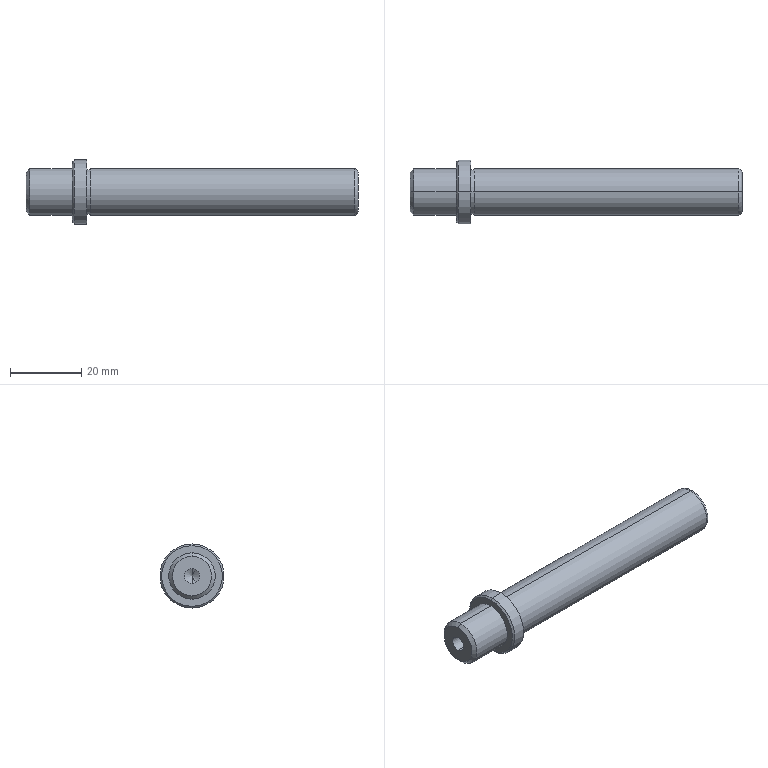Part | SolidWorks | features Chamfer 2, Fillet 1, HoleWzd 1, Revolution 1 | 1 solid | 23 faces | box 93 x 18 x 18 mm | volume 12586 mm3 | cylinder 10 | cone 6 | plane 5 | torus 2 | commonest cylinder face diameters 13 x4 4.2 x2 12.5 x2 18 x2
STEP:
#1=CARTESIAN_POINT('',(14.,0.,-2.1));
#2=VERTEX_POINT('',#1);
#3=CARTESIAN_POINT('',(14.,0.,2.1));
#4=VERTEX_POINT('',#3);
#5=CARTESIAN_POINT('',(14.,0.,0.));
#6=DIRECTION('',(-1.,0.,0.));
#7=DIRECTION('',(0.,0.,1.));
#8=AXIS2_PLACEMENT_3D('',#5,#6,#7);
#9=CIRCLE('',#8,2.1);
#10=EDGE_CURVE('',#2,#4,#9,.T.);
#11=ORIENTED_EDGE('',*,*,#10,.F.);
#12=CARTESIAN_POINT('',(0.,0.,-2.1));
#13=VERTEX_POINT('',#12);
#14=CARTESIAN_POINT('',(0.,0.,-2.1));
#15=DIRECTION('',(-1.,0.,0.));
#16=VECTOR('',#15,1000.);
#17=LINE('',#14,#16);
#18=EDGE_CURVE('',#2,#13,#17,.T.);
#19=ORIENTED_EDGE('',*,*,#18,.T.);
#20=CARTESIAN_POINT('',(0.,0.,2.1));
#21=VERTEX_POINT('',#20);
#22=CARTESIAN_POINT('',(0.,0.,0.));
#23=DIRECTION('',(-1.,0.,0.));
#24=DIRECTION('',(0.,0.,1.));
#25=AXIS2_PLACEMENT_3D('',#22,#23,#24);
#26=CIRCLE('',#25,2.1);
#27=EDGE_CURVE('',#13,#21,#26,.T.);
#28=ORIENTED_EDGE('',*,*,#27,.T.);
#29=CARTESIAN_POINT('',(0.,0.,2.1));
#30=DIRECTION('',(-1.,0.,0.));
#31=VECTOR('',#30,1000.);
#32=LINE('',#29,#31);
#33=EDGE_CURVE('',#4,#21,#32,.T.);
#34=ORIENTED_EDGE('',*,*,#33,.F.);
#35=EDGE_LOOP('',(#11,#19,#28,#34));
#36=FACE_OUTER_BOUND('',#35,.T.);
#37=CARTESIAN_POINT('',(0.,0.,0.));
#38=DIRECTION('',(-1.,0.,0.));
#39=DIRECTION('',(0.,0.,1.));
#40=AXIS2_PLACEMENT_3D('',#37,#38,#39);
#41=CYLINDRICAL_SURFACE('',#40,2.1);
#42=ADVANCED_FACE('',(#36),#41,.F.);
#43=CARTESIAN_POINT('',(15.262,0.,0.));
#44=VERTEX_POINT('',#43);
#45=CARTESIAN_POINT('',(14.,0.,2.1));
#46=DIRECTION('',(-0.515,0.,0.8572));
#47=VECTOR('',#46,1000.);
#48=LINE('',#45,#47);
#49=EDGE_CURVE('',#44,#4,#48,.T.);
#50=ORIENTED_EDGE('',*,*,#49,.F.);
#51=CARTESIAN_POINT('',(14.,0.,-2.1));
#52=DIRECTION('',(-0.515,0.,-0.8572));
#53=VECTOR('',#52,1000.);
#54=LINE('',#51,#53);
#55=EDGE_CURVE('',#44,#2,#54,.T.);
#56=ORIENTED_EDGE('',*,*,#55,.T.);
#57=ORIENTED_EDGE('',*,*,#10,.T.);
#58=EDGE_LOOP('',(#50,#56,#57));
#59=FACE_OUTER_BOUND('',#58,.T.);
#60=CARTESIAN_POINT('',(14.,0.,0.));
#61=DIRECTION('',(-1.,0.,0.));
#62=DIRECTION('',(0.,0.,1.));
#63=AXIS2_PLACEMENT_3D('',#60,#61,#62);
#64=CONICAL_SURFACE('',#63,2.1,1.03);
#65=ADVANCED_FACE('',(#59),#64,.F.);
#66=CARTESIAN_POINT('',(0.,0.,5.5));
#67=VERTEX_POINT('',#66);
#68=CARTESIAN_POINT('',(0.,0.,-5.5));
#69=VERTEX_POINT('',#68);
#70=CARTESIAN_POINT('',(0.,0.,0.));
#71=DIRECTION('',(-1.,0.,0.));
#72=DIRECTION('',(0.,0.,-1.));
#73=AXIS2_PLACEMENT_3D('',#70,#71,#72);
#74=CIRCLE('',#73,5.5);
#75=EDGE_CURVE('',#67,#69,#74,.T.);
#76=ORIENTED_EDGE('',*,*,#75,.F.);
#77=CARTESIAN_POINT('',(1.,0.,6.5));
#78=VERTEX_POINT('',#77);
#79=CARTESIAN_POINT('',(0.,0.,5.5));
#80=DIRECTION('',(0.7071,0.,0.7071));
#81=VECTOR('',#80,1000.);
#82=LINE('',#79,#81);
#83=EDGE_CURVE('',#67,#78,#82,.T.);
#84=ORIENTED_EDGE('',*,*,#83,.T.);
#85=CARTESIAN_POINT('',(1.,0.,-6.5));
#86=VERTEX_POINT('',#85);
#87=CARTESIAN_POINT('',(1.,0.,0.));
#88=DIRECTION('',(1.,0.,0.));
#89=DIRECTION('',(0.,0.,-1.));
#90=AXIS2_PLACEMENT_3D('',#87,#88,#89);
#91=CIRCLE('',#90,6.5);
#92=EDGE_CURVE('',#86,#78,#91,.T.);
#93=ORIENTED_EDGE('',*,*,#92,.F.);
#94=CARTESIAN_POINT('',(0.,0.,-5.5));
#95=DIRECTION('',(0.7071,0.,-0.7071));
#96=VECTOR('',#95,1000.);
#97=LINE('',#94,#96);
#98=EDGE_CURVE('',#69,#86,#97,.T.);
#99=ORIENTED_EDGE('',*,*,#98,.F.);
#100=EDGE_LOOP('',(#76,#84,#93,#99));
#101=FACE_OUTER_BOUND('',#100,.T.);
#102=CARTESIAN_POINT('',(0.,0.,0.));
#103=DIRECTION('',(1.,0.,0.));
#104=DIRECTION('',(0.,0.,-1.));
#105=AXIS2_PLACEMENT_3D('',#102,#103,#104);
#106=CONICAL_SURFACE('',#105,5.5,0.7854);
#107=ADVANCED_FACE('',(#101),#106,.T.);
#108=CARTESIAN_POINT('',(13.,0.,8.5));
#109=VERTEX_POINT('',#108);
#110=CARTESIAN_POINT('',(13.,0.,-8.5));
#111=VERTEX_POINT('',#110);
#112=CARTESIAN_POINT('',(13.,0.,0.));
#113=DIRECTION('',(-1.,0.,0.));
#114=DIRECTION('',(0.,0.,-1.));
#115=AXIS2_PLACEMENT_3D('',#112,#113,#114);
#116=CIRCLE('',#115,8.5);
#117=EDGE_CURVE('',#109,#111,#116,.T.);
#118=ORIENTED_EDGE('',*,*,#117,.F.);
#119=CARTESIAN_POINT('',(13.5,0.,9.));
#120=VERTEX_POINT('',#119);
#121=CARTESIAN_POINT('',(13.,0.,8.5));
#122=DIRECTION('',(0.7071,0.,0.7071));
#123=VECTOR('',#122,1000.);
#124=LINE('',#121,#123);
#125=EDGE_CURVE('',#109,#120,#124,.T.);
#126=ORIENTED_EDGE('',*,*,#125,.T.);
#127=CARTESIAN_POINT('',(13.5,0.,-9.));
#128=VERTEX_POINT('',#127);
#129=CARTESIAN_POINT('',(13.5,0.,0.));
#130=DIRECTION('',(1.,0.,0.));
#131=DIRECTION('',(0.,0.,-1.));
#132=AXIS2_PLACEMENT_3D('',#129,#130,#131);
#133=CIRCLE('',#132,9.);
#134=EDGE_CURVE('',#128,#120,#133,.T.);
#135=ORIENTED_EDGE('',*,*,#134,.F.);
#136=CARTESIAN_POINT('',(13.,0.,-8.5));
#137=DIRECTION('',(0.7071,0.,-0.7071));
#138=VECTOR('',#137,1000.);
#139=LINE('',#136,#138);
#140=EDGE_CURVE('',#111,#128,#139,.T.);
#141=ORIENTED_EDGE('',*,*,#140,.F.);
#142=EDGE_LOOP('',(#118,#126,#135,#141));
#143=FACE_OUTER_BOUND('',#142,.T.);
#144=CARTESIAN_POINT('',(13.,0.,0.));
#145=DIRECTION('',(1.,0.,0.));
#146=DIRECTION('',(0.,0.,-1.));
#147=AXIS2_PLACEMENT_3D('',#144,#145,#146);
#148=CONICAL_SURFACE('',#147,8.5,0.7854);
#149=ADVANCED_FACE('',(#143),#148,.T.);
#150=CARTESIAN_POINT('',(93.,0.,-5.5));
#151=VERTEX_POINT('',#150);
#152=CARTESIAN_POINT('',(93.,0.,5.5));
#153=VERTEX_POINT('',#152);
#154=CARTESIAN_POINT('',(93.,0.,0.));
#155=DIRECTION('',(1.,0.,0.));
#156=DIRECTION('',(0.,0.,1.));
#157=AXIS2_PLACEMENT_3D('',#154,#155,#156);
#158=CIRCLE('',#157,5.5);
#159=EDGE_CURVE('',#151,#153,#158,.T.);
#160=ORIENTED_EDGE('',*,*,#159,.F.);
#161=CARTESIAN_POINT('',(92.,0.,-6.5));
#162=VERTEX_POINT('',#161);
#163=CARTESIAN_POINT('',(92.,0.,-5.5));
#164=DIRECTION('',(0.,1.,0.));
#165=DIRECTION('',(0.,0.,1.));
#166=AXIS2_PLACEMENT_3D('',#163,#164,#165);
#167=CIRCLE('',#166,1.);
#168=EDGE_CURVE('',#151,#162,#167,.T.);
#169=ORIENTED_EDGE('',*,*,#168,.T.);
#170=CARTESIAN_POINT('',(92.,0.,6.5));
#171=VERTEX_POINT('',#170);
#172=CARTESIAN_POINT('',(92.,0.,0.));
#173=DIRECTION('',(-1.,0.,0.));
#174=DIRECTION('',(0.,0.,1.));
#175=AXIS2_PLACEMENT_3D('',#172,#173,#174);
#176=CIRCLE('',#175,6.5);
#177=EDGE_CURVE('',#171,#162,#176,.T.);
#178=ORIENTED_EDGE('',*,*,#177,.F.);
#179=CARTESIAN_POINT('',(92.,0.,5.5));
#180=DIRECTION('',(0.,-1.,0.));
#181=DIRECTION('',(0.,0.,-1.));
#182=AXIS2_PLACEMENT_3D('',#179,#180,#181);
#183=CIRCLE('',#182,1.);
#184=EDGE_CURVE('',#153,#171,#183,.T.);
#185=ORIENTED_EDGE('',*,*,#184,.F.);
#186=EDGE_LOOP('',(#160,#169,#178,#185));
#187=FACE_OUTER_BOUND('',#186,.T.);
#188=CARTESIAN_POINT('',(92.,0.,0.));
#189=DIRECTION('',(-1.,0.,0.));
#190=DIRECTION('',(0.,0.,1.));
#191=AXIS2_PLACEMENT_3D('',#188,#189,#190);
#192=TOROIDAL_SURFACE('',#191,5.5,1.);
#193=ADVANCED_FACE('',(#187),#192,.T.);
#194=CARTESIAN_POINT('',(17.,0.,9.));
#195=VERTEX_POINT('',#194);
#196=CARTESIAN_POINT('',(17.,0.,-9.));
#197=VERTEX_POINT('',#196);
#198=CARTESIAN_POINT('',(17.,0.,0.));
#199=DIRECTION('',(-1.,0.,0.));
#200=DIRECTION('',(0.,0.,1.));
#201=AXIS2_PLACEMENT_3D('',#198,#199,#200);
#202=CIRCLE('',#201,9.);
#203=EDGE_CURVE('',#195,#197,#202,.T.);
#204=ORIENTED_EDGE('',*,*,#203,.T.);
#205=CARTESIAN_POINT('',(0.,0.,-9.));
#206=DIRECTION('',(-1.,0.,0.));
#207=VECTOR('',#206,1000.);
#208=LINE('',#205,#207);
#209=EDGE_CURVE('',#197,#128,#208,.T.);
#210=ORIENTED_EDGE('',*,*,#209,.T.);
#211=ORIENTED_EDGE('',*,*,#134,.T.);
#212=CARTESIAN_POINT('',(0.,0.,9.));
#213=DIRECTION('',(-1.,0.,0.));
#214=VECTOR('',#213,1000.);
#215=LINE('',#212,#214);
#216=EDGE_CURVE('',#195,#120,#215,.T.);
#217=ORIENTED_EDGE('',*,*,#216,.F.);
#218=EDGE_LOOP('',(#204,#210,#211,#217));
#219=FACE_OUTER_BOUND('',#218,.T.);
#220=CARTESIAN_POINT('',(0.,0.,0.));
#221=DIRECTION('',(-1.,0.,0.));
#222=DIRECTION('',(0.,0.,1.));
#223=AXIS2_PLACEMENT_3D('',#220,#221,#222);
#224=CYLINDRICAL_SURFACE('',#223,9.);
#225=ADVANCED_FACE('',(#219),#224,.T.);
#226=CARTESIAN_POINT('',(18.,0.,6.25));
#227=VERTEX_POINT('',#226);
#228=CARTESIAN_POINT('',(18.,0.,-6.25));
#229=VERTEX_POINT('',#228);
#230=CARTESIAN_POINT('',(18.,0.,0.));
#231=DIRECTION('',(-1.,0.,0.));
#232=DIRECTION('',(0.,0.,1.));
#233=AXIS2_PLACEMENT_3D('',#230,#231,#232);
#234=CIRCLE('',#233,6.25);
#235=EDGE_CURVE('',#227,#229,#234,.T.);
#236=ORIENTED_EDGE('',*,*,#235,.T.);
#237=CARTESIAN_POINT('',(17.,0.,-6.25));
#238=VERTEX_POINT('',#237);
#239=CARTESIAN_POINT('',(0.,0.,-6.25));
#240=DIRECTION('',(-1.,0.,0.));
#241=VECTOR('',#240,1000.);
#242=LINE('',#239,#241);
#243=EDGE_CURVE('',#229,#238,#242,.T.);
#244=ORIENTED_EDGE('',*,*,#243,.T.);
#245=CARTESIAN_POINT('',(17.,0.,6.25));
#246=VERTEX_POINT('',#245);
#247=CARTESIAN_POINT('',(17.,0.,0.));
#248=DIRECTION('',(-1.,0.,0.));
#249=DIRECTION('',(0.,0.,1.));
#250=AXIS2_PLACEMENT_3D('',#247,#248,#249);
#251=CIRCLE('',#250,6.25);
#252=EDGE_CURVE('',#246,#238,#251,.T.);
#253=ORIENTED_EDGE('',*,*,#252,.F.);
#254=CARTESIAN_POINT('',(0.,0.,6.25));
#255=DIRECTION('',(-1.,0.,0.));
#256=VECTOR('',#255,1000.);
#257=LINE('',#254,#256);
#258=EDGE_CURVE('',#227,#246,#257,.T.);
#259=ORIENTED_EDGE('',*,*,#258,.F.);
#260=EDGE_LOOP('',(#236,#244,#253,#259));
#261=FACE_OUTER_BOUND('',#260,.T.);
#262=CARTESIAN_POINT('',(0.,0.,0.));
#263=DIRECTION('',(-1.,0.,0.));
#264=DIRECTION('',(0.,0.,1.));
#265=AXIS2_PLACEMENT_3D('',#262,#263,#264);
#266=CYLINDRICAL_SURFACE('',#265,6.25);
#267=ADVANCED_FACE('',(#261),#266,.T.);
#268=ORIENTED_EDGE('',*,*,#177,.T.);
#269=CARTESIAN_POINT('',(18.,0.,-6.5));
#270=VERTEX_POINT('',#269);
#271=CARTESIAN_POINT('',(0.,0.,-6.5));
#272=DIRECTION('',(-1.,0.,0.));
#273=VECTOR('',#272,1000.);
#274=LINE('',#271,#273);
#275=EDGE_CURVE('',#162,#270,#274,.T.);
#276=ORIENTED_EDGE('',*,*,#275,.T.);
#277=CARTESIAN_POINT('',(18.,0.,6.5));
#278=VERTEX_POINT('',#277);
#279=CARTESIAN_POINT('',(18.,0.,0.));
#280=DIRECTION('',(-1.,0.,0.));
#281=DIRECTION('',(0.,0.,1.));
#282=AXIS2_PLACEMENT_3D('',#279,#280,#281);
#283=CIRCLE('',#282,6.5);
#284=EDGE_CURVE('',#278,#270,#283,.T.);
#285=ORIENTED_EDGE('',*,*,#284,.F.);
#286=CARTESIAN_POINT('',(0.,0.,6.5));
#287=DIRECTION('',(-1.,0.,0.));
#288=VECTOR('',#287,1000.);
#289=LINE('',#286,#288);
#290=EDGE_CURVE('',#171,#278,#289,.T.);
#291=ORIENTED_EDGE('',*,*,#290,.F.);
#292=EDGE_LOOP('',(#268,#276,#285,#291));
#293=FACE_OUTER_BOUND('',#292,.T.);
#294=CARTESIAN_POINT('',(0.,0.,0.));
#295=DIRECTION('',(-1.,0.,0.));
#296=DIRECTION('',(0.,0.,1.));
#297=AXIS2_PLACEMENT_3D('',#294,#295,#296);
#298=CYLINDRICAL_SURFACE('',#297,6.5);
#299=ADVANCED_FACE('',(#293),#298,.T.);
#300=CARTESIAN_POINT('',(13.,0.,6.5));
#301=VERTEX_POINT('',#300);
#302=CARTESIAN_POINT('',(13.,0.,-6.5));
#303=VERTEX_POINT('',#302);
#304=CARTESIAN_POINT('',(13.,0.,0.));
#305=DIRECTION('',(-1.,0.,0.));
#306=DIRECTION('',(0.,0.,1.));
#307=AXIS2_PLACEMENT_3D('',#304,#305,#306);
#308=CIRCLE('',#307,6.5);
#309=EDGE_CURVE('',#301,#303,#308,.T.);
#310=ORIENTED_EDGE('',*,*,#309,.T.);
#311=CARTESIAN_POINT('',(0.,0.,-6.5));
#312=DIRECTION('',(-1.,0.,0.));
#313=VECTOR('',#312,1000.);
#314=LINE('',#311,#313);
#315=EDGE_CURVE('',#303,#86,#314,.T.);
#316=ORIENTED_EDGE('',*,*,#315,.T.);
#317=ORIENTED_EDGE('',*,*,#92,.T.);
#318=CARTESIAN_POINT('',(0.,0.,6.5));
#319=DIRECTION('',(-1.,0.,0.));
#320=VECTOR('',#319,1000.);
#321=LINE('',#318,#320);
#322=EDGE_CURVE('',#301,#78,#321,.T.);
#323=ORIENTED_EDGE('',*,*,#322,.F.);
#324=EDGE_LOOP('',(#310,#316,#317,#323));
#325=FACE_OUTER_BOUND('',#324,.T.);
#326=CARTESIAN_POINT('',(0.,0.,0.));
#327=DIRECTION('',(-1.,0.,0.));
#328=DIRECTION('',(0.,0.,1.));
#329=AXIS2_PLACEMENT_3D('',#326,#327,#328);
#330=CYLINDRICAL_SURFACE('',#329,6.5);
#331=ADVANCED_FACE('',(#325),#330,.T.);
#332=ORIENTED_EDGE('',*,*,#315,.F.);
#333=CARTESIAN_POINT('',(13.,0.,0.));
#334=DIRECTION('',(-1.,0.,0.));
#335=DIRECTION('',(0.,0.,1.));
#336=AXIS2_PLACEMENT_3D('',#333,#334,#335);
#337=CIRCLE('',#336,6.5);
#338=EDGE_CURVE('',#303,#301,#337,.T.);
#339=ORIENTED_EDGE('',*,*,#338,.T.);
#340=ORIENTED_EDGE('',*,*,#322,.T.);
#341=CARTESIAN_POINT('',(1.,0.,0.));
#342=DIRECTION('',(1.,0.,0.));
#343=DIRECTION('',(0.,0.,-1.));
#344=AXIS2_PLACEMENT_3D('',#341,#342,#343);
#345=CIRCLE('',#344,6.5);
#346=EDGE_CURVE('',#78,#86,#345,.T.);
#347=ORIENTED_EDGE('',*,*,#346,.T.);
#348=EDGE_LOOP('',(#332,#339,#340,#347));
#349=FACE_OUTER_BOUND('',#348,.T.);
#350=CARTESIAN_POINT('',(0.,0.,0.));
#351=DIRECTION('',(-1.,0.,0.));
#352=DIRECTION('',(0.,0.,1.));
#353=AXIS2_PLACEMENT_3D('',#350,#351,#352);
#354=CYLINDRICAL_SURFACE('',#353,6.5);
#355=ADVANCED_FACE('',(#349),#354,.T.);
#356=CARTESIAN_POINT('',(0.,0.,0.));
#357=DIRECTION('',(-1.,0.,0.));
#358=DIRECTION('',(0.,0.,1.));
#359=AXIS2_PLACEMENT_3D('',#356,#357,#358);
#360=CIRCLE('',#359,2.1);
#361=EDGE_CURVE('',#21,#13,#360,.T.);
#362=ORIENTED_EDGE('',*,*,#361,.F.);
#363=ORIENTED_EDGE('',*,*,#27,.F.);
#364=EDGE_LOOP('',(#362,#363));
#365=FACE_BOUND('',#364,.T.);
#366=CARTESIAN_POINT('',(0.,0.,0.));
#367=DIRECTION('',(-1.,0.,0.));
#368=DIRECTION('',(0.,0.,-1.));
#369=AXIS2_PLACEMENT_3D('',#366,#367,#368);
#370=CIRCLE('',#369,5.5);
#371=EDGE_CURVE('',#69,#67,#370,.T.);
#372=ORIENTED_EDGE('',*,*,#371,.T.);
#373=ORIENTED_EDGE('',*,*,#75,.T.);
#374=EDGE_LOOP('',(#372,#373));
#375=FACE_OUTER_BOUND('',#374,.T.);
#376=CARTESIAN_POINT('',(0.,6.5,0.));
#377=DIRECTION('',(1.,0.,0.));
#378=DIRECTION('',(0.,0.,-1.));
#379=AXIS2_PLACEMENT_3D('',#376,#377,#378);
#380=PLANE('',#379);
#381=ADVANCED_FACE('',(#365,#375),#380,.F.);
#382=CARTESIAN_POINT('',(93.,0.,0.));
#383=DIRECTION('',(1.,0.,0.));
#384=DIRECTION('',(0.,0.,1.));
#385=AXIS2_PLACEMENT_3D('',#382,#383,#384);
#386=CIRCLE('',#385,5.5);
#387=EDGE_CURVE('',#153,#151,#386,.T.);
#388=ORIENTED_EDGE('',*,*,#387,.T.);
#389=ORIENTED_EDGE('',*,*,#159,.T.);
#390=EDGE_LOOP('',(#388,#389));
#391=FACE_OUTER_BOUND('',#390,.T.);
#392=CARTESIAN_POINT('',(93.,6.5,0.));
#393=DIRECTION('',(-1.,0.,0.));
#394=DIRECTION('',(0.,0.,1.));
#395=AXIS2_PLACEMENT_3D('',#392,#393,#394);
#396=PLANE('',#395);
#397=ADVANCED_FACE('',(#391),#396,.F.);
#398=ORIENTED_EDGE('',*,*,#275,.F.);
#399=CARTESIAN_POINT('',(92.,0.,0.));
#400=DIRECTION('',(-1.,0.,0.));
#401=DIRECTION('',(0.,0.,1.));
#402=AXIS2_PLACEMENT_3D('',#399,#400,#401);
#403=CIRCLE('',#402,6.5);
#404=EDGE_CURVE('',#162,#171,#403,.T.);
#405=ORIENTED_EDGE('',*,*,#404,.T.);
#406=ORIENTED_EDGE('',*,*,#290,.T.);
#407=CARTESIAN_POINT('',(18.,0.,0.));
#408=DIRECTION('',(-1.,0.,0.));
#409=DIRECTION('',(0.,0.,1.));
#410=AXIS2_PLACEMENT_3D('',#407,#408,#409);
#411=CIRCLE('',#410,6.5);
#412=EDGE_CURVE('',#270,#278,#411,.T.);
#413=ORIENTED_EDGE('',*,*,#412,.F.);
#414=EDGE_LOOP('',(#398,#405,#406,#413));
#415=FACE_OUTER_BOUND('',#414,.T.);
#416=CARTESIAN_POINT('',(0.,0.,0.));
#417=DIRECTION('',(-1.,0.,0.));
#418=DIRECTION('',(0.,0.,1.));
#419=AXIS2_PLACEMENT_3D('',#416,#417,#418);
#420=CYLINDRICAL_SURFACE('',#419,6.5);
#421=ADVANCED_FACE('',(#415),#420,.T.);
#422=ORIENTED_EDGE('',*,*,#235,.F.);
#423=CARTESIAN_POINT('',(18.,0.,0.));
#424=DIRECTION('',(-1.,0.,0.));
#425=DIRECTION('',(0.,0.,1.));
#426=AXIS2_PLACEMENT_3D('',#423,#424,#425);
#427=CIRCLE('',#426,6.25);
#428=EDGE_CURVE('',#229,#227,#427,.T.);
#429=ORIENTED_EDGE('',*,*,#428,.F.);
#430=EDGE_LOOP('',(#422,#429));
#431=FACE_BOUND('',#430,.T.);
#432=ORIENTED_EDGE('',*,*,#284,.T.);
#433=ORIENTED_EDGE('',*,*,#412,.T.);
#434=EDGE_LOOP('',(#432,#433));
#435=FACE_OUTER_BOUND('',#434,.T.);
#436=CARTESIAN_POINT('',(18.,6.25,0.));
#437=DIRECTION('',(1.,0.,0.));
#438=DIRECTION('',(0.,0.,-1.));
#439=AXIS2_PLACEMENT_3D('',#436,#437,#438);
#440=PLANE('',#439);
#441=ADVANCED_FACE('',(#431,#435),#440,.F.);
#442=ORIENTED_EDGE('',*,*,#243,.F.);
#443=ORIENTED_EDGE('',*,*,#428,.T.);
#444=ORIENTED_EDGE('',*,*,#258,.T.);
#445=CARTESIAN_POINT('',(17.,0.,0.));
#446=DIRECTION('',(-1.,0.,0.));
#447=DIRECTION('',(0.,0.,1.));
#448=AXIS2_PLACEMENT_3D('',#445,#446,#447);
#449=CIRCLE('',#448,6.25);
#450=EDGE_CURVE('',#238,#246,#449,.T.);
#451=ORIENTED_EDGE('',*,*,#450,.F.);
#452=EDGE_LOOP('',(#442,#443,#444,#451));
#453=FACE_OUTER_BOUND('',#452,.T.);
#454=CARTESIAN_POINT('',(0.,0.,0.));
#455=DIRECTION('',(-1.,0.,0.));
#456=DIRECTION('',(0.,0.,1.));
#457=AXIS2_PLACEMENT_3D('',#454,#455,#456);
#458=CYLINDRICAL_SURFACE('',#457,6.25);
#459=ADVANCED_FACE('',(#453),#458,.T.);
#460=ORIENTED_EDGE('',*,*,#203,.F.);
#461=CARTESIAN_POINT('',(17.,0.,0.));
#462=DIRECTION('',(-1.,0.,0.));
#463=DIRECTION('',(0.,0.,1.));
#464=AXIS2_PLACEMENT_3D('',#461,#462,#463);
#465=CIRCLE('',#464,9.);
#466=EDGE_CURVE('',#197,#195,#465,.T.);
#467=ORIENTED_EDGE('',*,*,#466,.F.);
#468=EDGE_LOOP('',(#460,#467));
#469=FACE_OUTER_BOUND('',#468,.T.);
#470=ORIENTED_EDGE('',*,*,#252,.T.);
#471=ORIENTED_EDGE('',*,*,#450,.T.);
#472=EDGE_LOOP('',(#470,#471));
#473=FACE_BOUND('',#472,.T.);
#474=CARTESIAN_POINT('',(17.,9.,0.));
#475=DIRECTION('',(-1.,0.,0.));
#476=DIRECTION('',(0.,0.,1.));
#477=AXIS2_PLACEMENT_3D('',#474,#475,#476);
#478=PLANE('',#477);
#479=ADVANCED_FACE('',(#469,#473),#478,.F.);
#480=ORIENTED_EDGE('',*,*,#209,.F.);
#481=ORIENTED_EDGE('',*,*,#466,.T.);
#482=ORIENTED_EDGE('',*,*,#216,.T.);
#483=CARTESIAN_POINT('',(13.5,0.,0.));
#484=DIRECTION('',(1.,0.,0.));
#485=DIRECTION('',(0.,0.,-1.));
#486=AXIS2_PLACEMENT_3D('',#483,#484,#485);
#487=CIRCLE('',#486,9.);
#488=EDGE_CURVE('',#120,#128,#487,.T.);
#489=ORIENTED_EDGE('',*,*,#488,.T.);
#490=EDGE_LOOP('',(#480,#481,#482,#489));
#491=FACE_OUTER_BOUND('',#490,.T.);
#492=CARTESIAN_POINT('',(0.,0.,0.));
#493=DIRECTION('',(-1.,0.,0.));
#494=DIRECTION('',(0.,0.,1.));
#495=AXIS2_PLACEMENT_3D('',#492,#493,#494);
#496=CYLINDRICAL_SURFACE('',#495,9.);
#497=ADVANCED_FACE('',(#491),#496,.T.);
#498=CARTESIAN_POINT('',(13.,0.,0.));
#499=DIRECTION('',(-1.,0.,0.));
#500=DIRECTION('',(0.,0.,-1.));
#501=AXIS2_PLACEMENT_3D('',#498,#499,#500);
#502=CIRCLE('',#501,8.5);
#503=EDGE_CURVE('',#111,#109,#502,.T.);
#504=ORIENTED_EDGE('',*,*,#503,.T.);
#505=ORIENTED_EDGE('',*,*,#117,.T.);
#506=EDGE_LOOP('',(#504,#505));
#507=FACE_OUTER_BOUND('',#506,.T.);
#508=ORIENTED_EDGE('',*,*,#309,.F.);
#509=ORIENTED_EDGE('',*,*,#338,.F.);
#510=EDGE_LOOP('',(#508,#509));
#511=FACE_BOUND('',#510,.T.);
#512=CARTESIAN_POINT('',(13.,6.5,0.));
#513=DIRECTION('',(1.,0.,0.));
#514=DIRECTION('',(0.,0.,-1.));
#515=AXIS2_PLACEMENT_3D('',#512,#513,#514);
#516=PLANE('',#515);
#517=ADVANCED_FACE('',(#507,#511),#516,.F.);
#518=ORIENTED_EDGE('',*,*,#168,.F.);
#519=ORIENTED_EDGE('',*,*,#387,.F.);
#520=ORIENTED_EDGE('',*,*,#184,.T.);
#521=ORIENTED_EDGE('',*,*,#404,.F.);
#522=EDGE_LOOP('',(#518,#519,#520,#521));
#523=FACE_OUTER_BOUND('',#522,.T.);
#524=CARTESIAN_POINT('',(92.,0.,0.));
#525=DIRECTION('',(-1.,0.,0.));
#526=DIRECTION('',(0.,0.,1.));
#527=AXIS2_PLACEMENT_3D('',#524,#525,#526);
#528=TOROIDAL_SURFACE('',#527,5.5,1.);
#529=ADVANCED_FACE('',(#523),#528,.T.);
#530=ORIENTED_EDGE('',*,*,#125,.F.);
#531=ORIENTED_EDGE('',*,*,#503,.F.);
#532=ORIENTED_EDGE('',*,*,#140,.T.);
#533=ORIENTED_EDGE('',*,*,#488,.F.);
#534=EDGE_LOOP('',(#530,#531,#532,#533));
#535=FACE_OUTER_BOUND('',#534,.T.);
#536=CARTESIAN_POINT('',(13.,0.,0.));
#537=DIRECTION('',(1.,0.,0.));
#538=DIRECTION('',(0.,0.,-1.));
#539=AXIS2_PLACEMENT_3D('',#536,#537,#538);
#540=CONICAL_SURFACE('',#539,8.5,0.7854);
#541=ADVANCED_FACE('',(#535),#540,.T.);
#542=ORIENTED_EDGE('',*,*,#83,.F.);
#543=ORIENTED_EDGE('',*,*,#371,.F.);
#544=ORIENTED_EDGE('',*,*,#98,.T.);
#545=ORIENTED_EDGE('',*,*,#346,.F.);
#546=EDGE_LOOP('',(#542,#543,#544,#545));
#547=FACE_OUTER_BOUND('',#546,.T.);
#548=CARTESIAN_POINT('',(0.,0.,0.));
#549=DIRECTION('',(1.,0.,0.));
#550=DIRECTION('',(0.,0.,-1.));
#551=AXIS2_PLACEMENT_3D('',#548,#549,#550);
#552=CONICAL_SURFACE('',#551,5.5,0.7854);
#553=ADVANCED_FACE('',(#547),#552,.T.);
#554=ORIENTED_EDGE('',*,*,#55,.F.);
#555=ORIENTED_EDGE('',*,*,#49,.T.);
#556=CARTESIAN_POINT('',(14.,0.,0.));
#557=DIRECTION('',(-1.,0.,0.));
#558=DIRECTION('',(0.,0.,1.));
#559=AXIS2_PLACEMENT_3D('',#556,#557,#558);
#560=CIRCLE('',#559,2.1);
#561=EDGE_CURVE('',#4,#2,#560,.T.);
#562=ORIENTED_EDGE('',*,*,#561,.T.);
#563=EDGE_LOOP('',(#554,#555,#562));
#564=FACE_OUTER_BOUND('',#563,.T.);
#565=CARTESIAN_POINT('',(14.,0.,0.));
#566=DIRECTION('',(-1.,0.,0.));
#567=DIRECTION('',(0.,0.,1.));
#568=AXIS2_PLACEMENT_3D('',#565,#566,#567);
#569=CONICAL_SURFACE('',#568,2.1,1.03);
#570=ADVANCED_FACE('',(#564),#569,.F.);
#571=ORIENTED_EDGE('',*,*,#18,.F.);
#572=ORIENTED_EDGE('',*,*,#561,.F.);
#573=ORIENTED_EDGE('',*,*,#33,.T.);
#574=ORIENTED_EDGE('',*,*,#361,.T.);
#575=EDGE_LOOP('',(#571,#572,#573,#574));
#576=FACE_OUTER_BOUND('',#575,.T.);
#577=CARTESIAN_POINT('',(0.,0.,0.));
#578=DIRECTION('',(-1.,0.,0.));
#579=DIRECTION('',(0.,0.,1.));
#580=AXIS2_PLACEMENT_3D('',#577,#578,#579);
#581=CYLINDRICAL_SURFACE('',#580,2.1);
#582=ADVANCED_FACE('',(#576),#581,.F.);
#583=CLOSED_SHELL('',(#42,#65,#107,#149,#193,#225,#267,#299,#331,#355,#381,#397,#421,#441,#459,#479,#497,#517,#529,#541,#553,#570,#582));
#584=MANIFOLD_SOLID_BREP('',#583);
#585=CARTESIAN_POINT('',(0.,0.,0.));
#586=DIRECTION('',(0.,0.,1.));
#587=DIRECTION('',(1.,0.,0.));
#588=AXIS2_PLACEMENT_3D('',#585,#586,#587);
#589=(LENGTH_UNIT()NAMED_UNIT(*)SI_UNIT(.MILLI.,.METRE.));
#590=UNCERTAINTY_MEASURE_WITH_UNIT(LENGTH_MEASURE(0.00001),#589,'','');
#591=(NAMED_UNIT(*)PLANE_ANGLE_UNIT()SI_UNIT($,.RADIAN.));
#592=(NAMED_UNIT(*)SI_UNIT($,.STERADIAN.)SOLID_ANGLE_UNIT());
#593=(GEOMETRIC_REPRESENTATION_CONTEXT(3)GLOBAL_UNCERTAINTY_ASSIGNED_CONTEXT((#590))GLOBAL_UNIT_ASSIGNED_CONTEXT((#589,#591,#592))REPRESENTATION_CONTEXT('',''));
#594=ADVANCED_BREP_SHAPE_REPRESENTATION('',(#584,#588),#593);